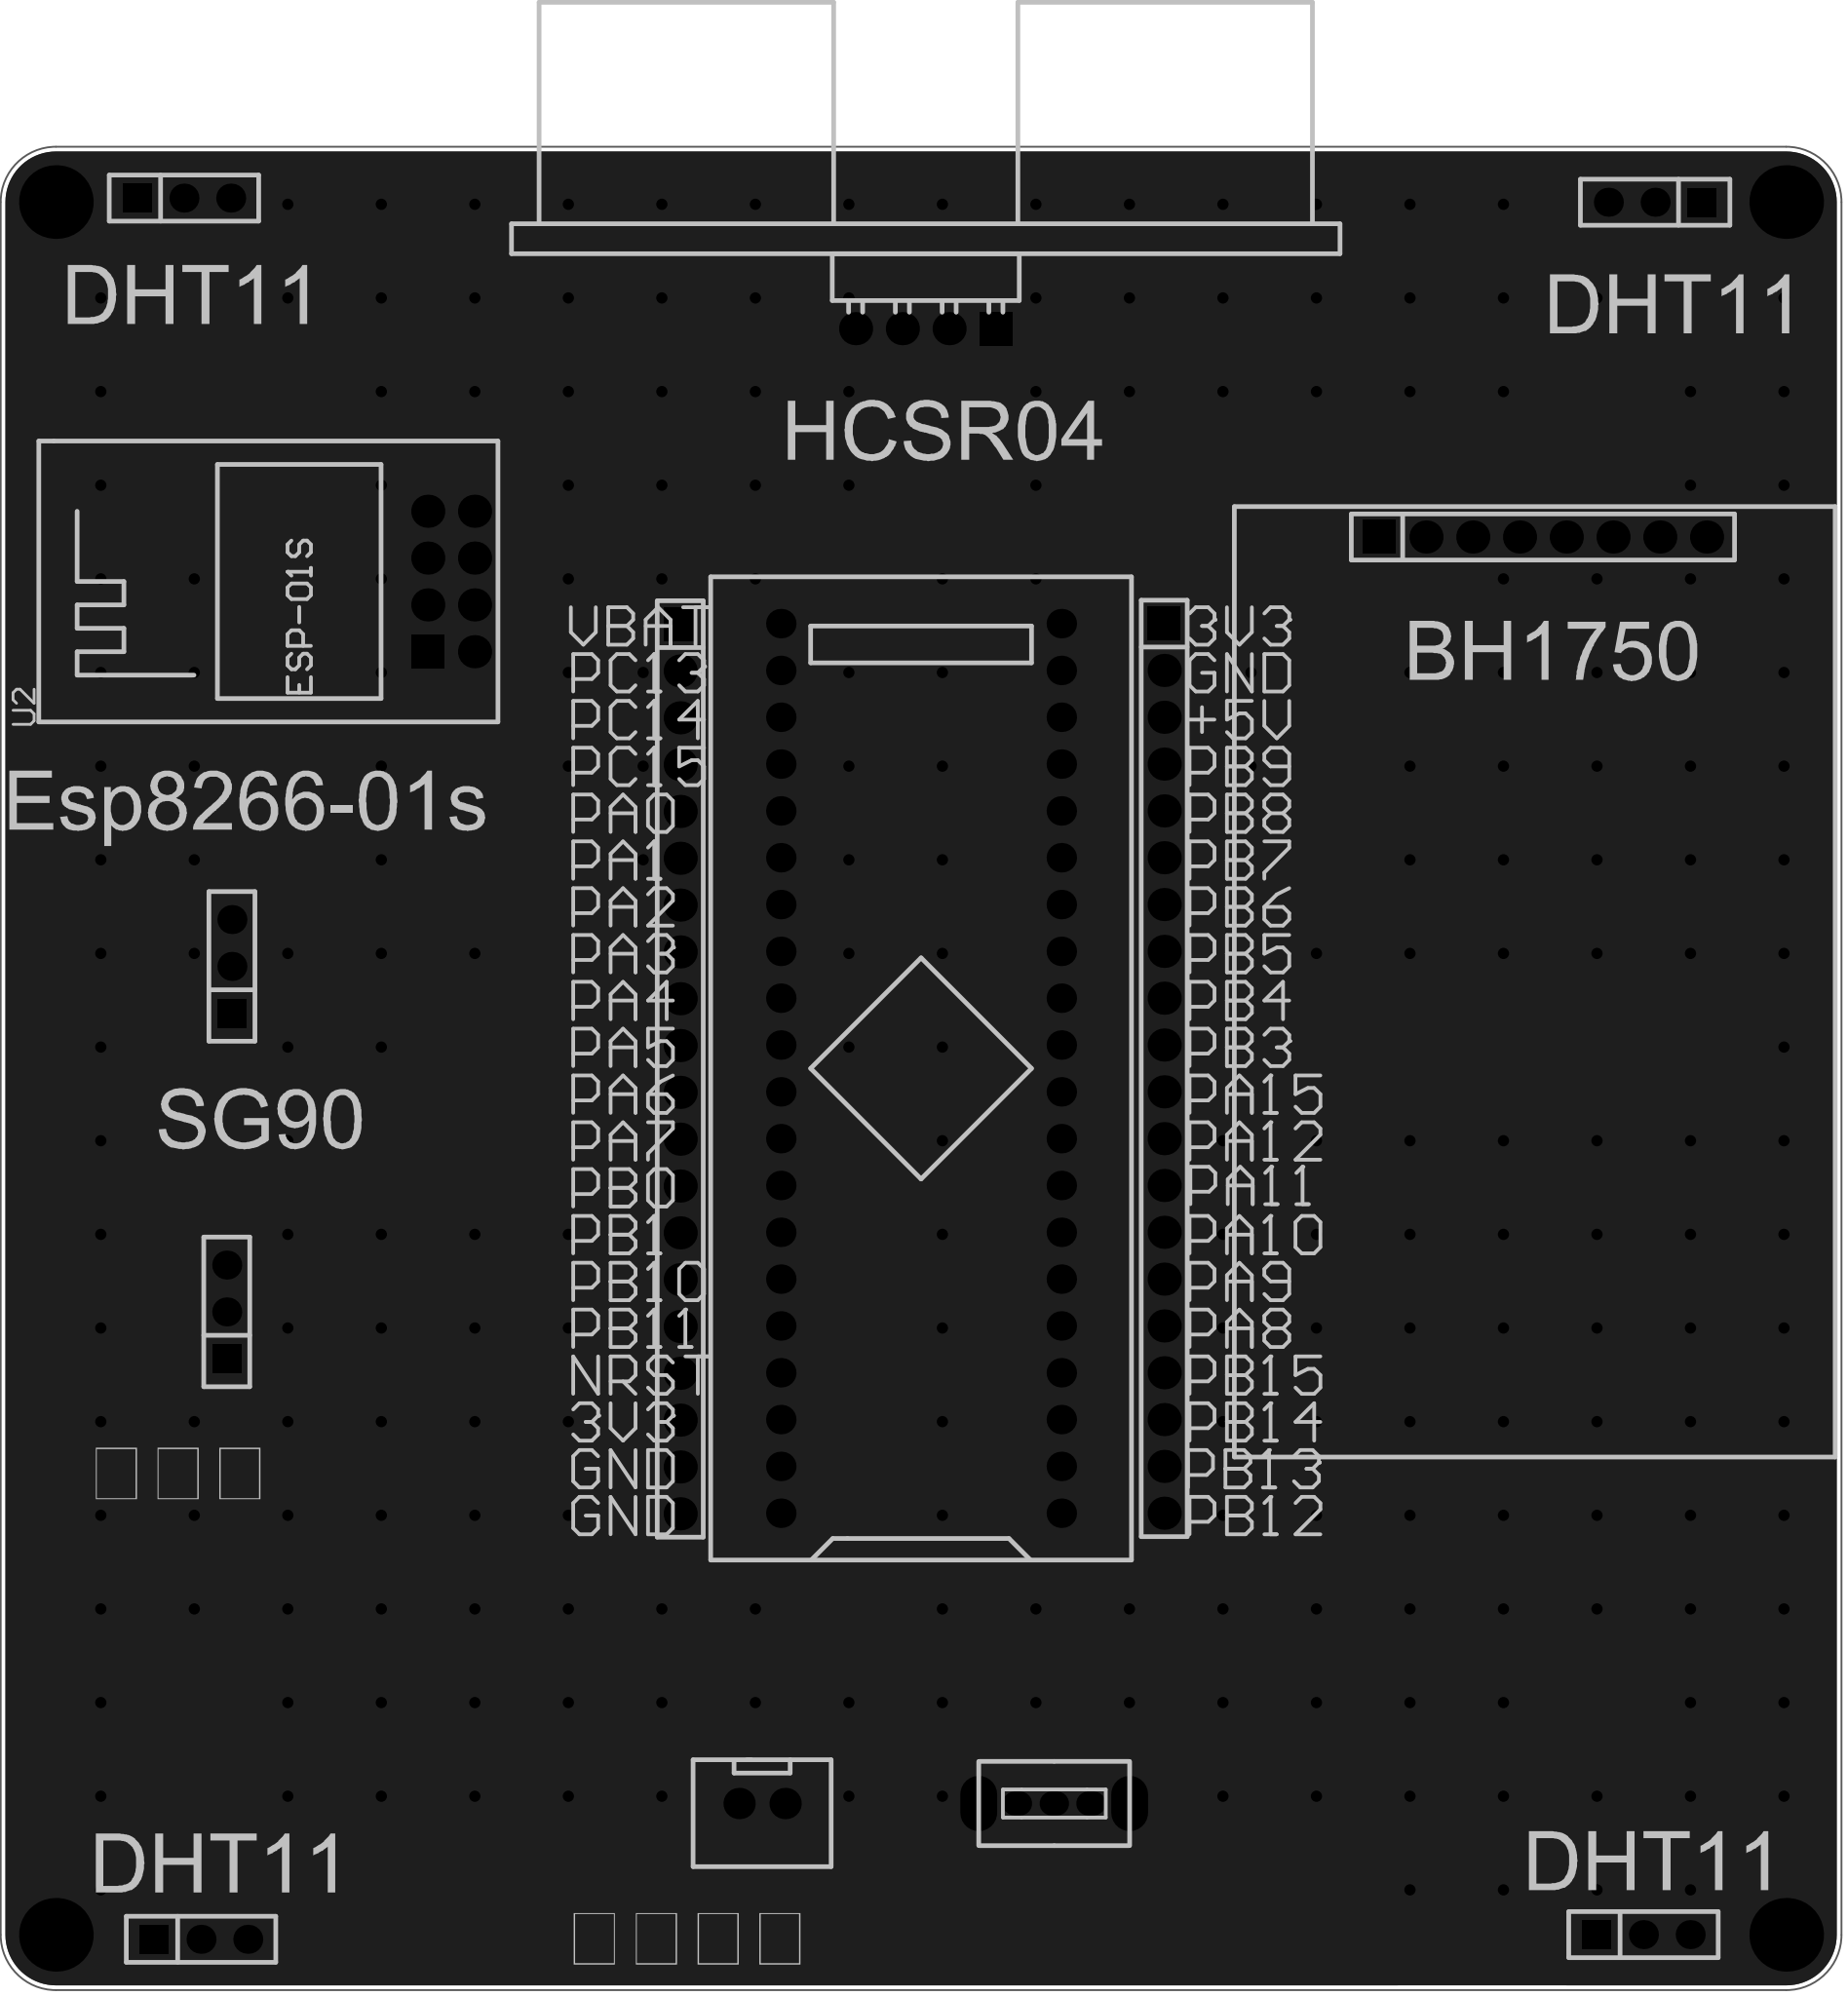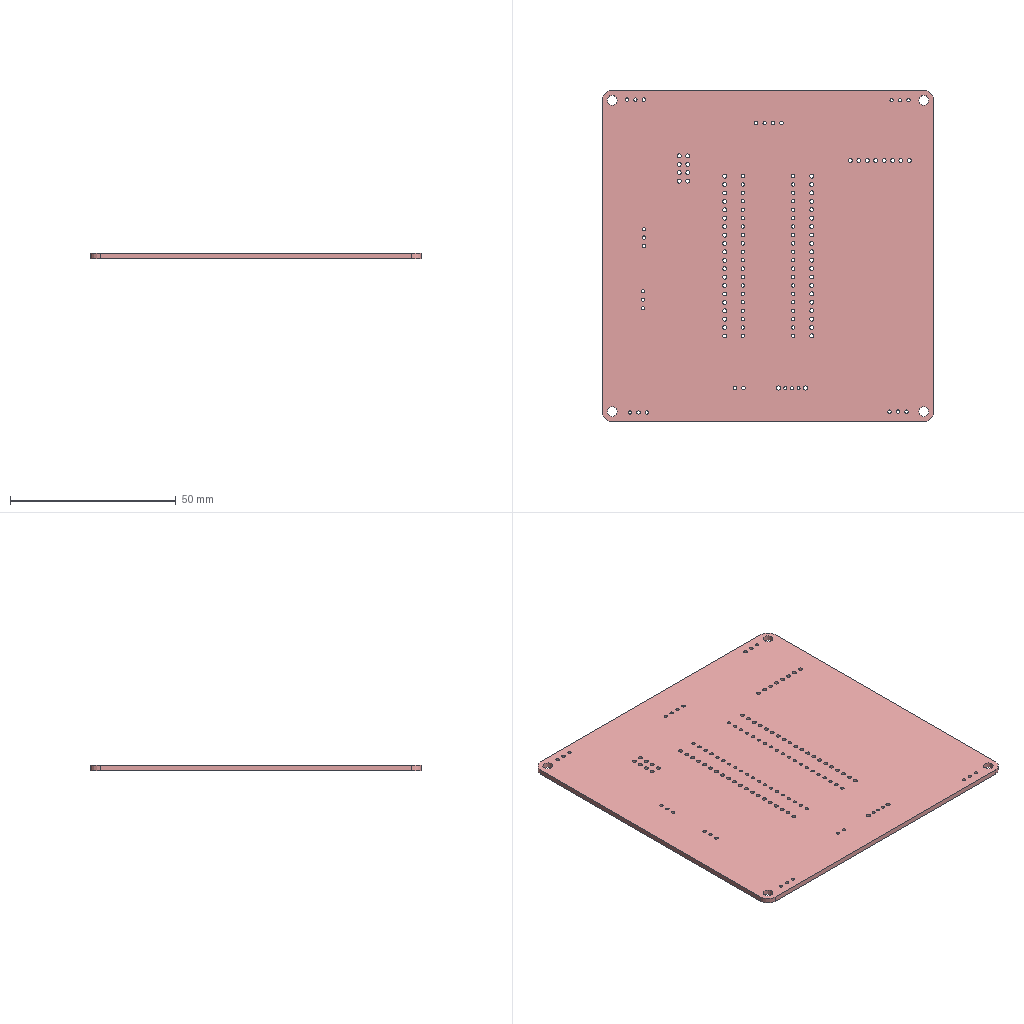Circuit board layout | Altium Designer | box 100 x 100 x 1.6 mm
Layer stack:
# Altium Designer layer stack of  (unit mm; dielectric type: 0 none, 1 core, 2 prepreg, 3 surface material)
index,name,kind,layer,copper_thickness_mm,dielectric_type,dielectric_thickness_mm,dielectric_material,dielectric_constant
0,Top Paste Mask Layer,other,,,,,,
1,Top Silkscreen Layer,other,,,,,,
2,Top Solder Mask Layer,dielectric,,,3,0.01,,3.3
3,Top Layer,copper,Top Layer,0.035,,,,
4,Dielectric1,dielectric,,,3,1.51,FR4,4.5
5,Bottom Layer,copper,Bottom Layer,0.035,,,,
6,Bottom Solder Mask Layer,dielectric,,,3,0.01,,3.3
7,Bottom Silkscreen Layer,other,,,,,,
8,Bottom Paste Mask Layer,other,,,,,,
# drill layer pairs: low layer,high layer
drill_pair,Top Layer,Bottom Layer
Part placement:
Designator,Comment,Layer,Footprint,Center-X(mm),Center-Y(mm),Rotation
U1,STM32F103C8T6-Card,TopLayer,CONN-TH_L53.3-W22.9_STM32F103C8T6-CARD,141.351,130.937,90
CN4,XH2.54*2P_直插,TopLayer,CONN-TH_2P-P2.50-XH2.54-2P,132.715,91.059,0
SW5,,TopLayer,拨动开关,148.582,91.059,180
H1,,TopLayer,HDR-TH_3P-P2.54-V-F,103.632,117.729,90
H3,,TopLayer,HDR-TH_3P-P2.54-V-F,181.229,177.927,180
U2,ESP-01S,TopLayer,WIFIM-TH_ESP-01S,115.824,157.353,90
H2,,TopLayer,HDR-TH_3P-P2.54-V-F,180.594,83.947,0
H4,,TopLayer,HDR-TH_3P-P2.54-V-F,101.307,178.151,0
U3,HC-SR04,TopLayer,TH_HC-SR04V,141.605,171.069,180
H5,,TopLayer,HDR-TH_8P-P2.54-V-F-1,175.133,159.766,0
H7,,TopLayer,HDR-TH_3P-P2.54-V-F,102.235,83.693,0
H8,,TopLayer,HDR-TH_3P-P2.54-V-F,103.912,136.472,90
H6,,TopLayer,HDR-TH_20P-P2.54-V-M-1,128.267,130.907,270
H9,,TopLayer,HDR-TH_20P-P2.54-V-M-1,154.559,130.937,270
Pad and via stacks:
# Altium Designer via and pad stacks of  (unit mm). Each distinct definition once, with the count of objects using it.
# via: kind,start_layer,end_layer,hole_mm,diameter_mm,mode(0 simple;1 top-mid-bottom;2 full stack),diameter_per_layer,count,example_net
# pad: kind,layer,hole_mm,hole_type(0 round;1 square;2 slot),plating,top_size,top_shape(1 round;2 rect;3 octagon;9 rounded rect),mid_size,bottom_size,mode,footprint,size_per_layer,count,example
pad,Multi-Layer,3,0,plated,4x4,1,4x4,4x4,0,,,4,1
pad,Multi-Layer,1,0,plated,1.6x1.6,1,1.6x1.6,1.6x1.6,0,CONN-TH_L53.3-W22.9_STM32F103C8T6-CARD,,40,U1.1
pad,Multi-Layer,1.05,0,plated,1.7x1.7,1,1.7x1.7,1.7x1.7,0,CONN-TH_2P-P2.50-XH2.54-2P,,2,CN4.2
pad,Multi-Layer,0.8992,0,plated,1.6x1.3,1,1.6x1.3,1.6x1.3,0,\u00B2\u00A6\u00B6\u00AF\u00BF\u00AA\u00B9\u00D8,,3,SW5.1
pad,Multi-Layer,1.3,0,plated,3x1.999,1,3x1.999,3x1.999,0,\u00B2\u00A6\u00B6\u00AF\u00BF\u00AA\u00B9\u00D8,,2,SW5.4
pad,Multi-Layer,1.02,0,plated,1.575x1.575,1,1.575x1.575,1.575x1.575,0,HDR-TH_3P-P2.54-V-F,,12,H1.3
pad,Multi-Layer,1.02,0,plated,1.575x1.575,2,1.575x1.575,1.575x1.575,0,HDR-TH_3P-P2.54-V-F,,6,H1.1
pad,Multi-Layer,1.2,0,plated,1.8x1.8,2,1.8x1.8,1.8x1.8,0,WIFIM-TH_ESP-01S,,1,U2.1
pad,Multi-Layer,1.2,0,plated,1.8x1.8,1,1.8x1.8,1.8x1.8,0,WIFIM-TH_ESP-01S,,7,U2.2
pad,Multi-Layer,1.001,0,plated,1.8x1.8,1,1.8x1.8,1.8x1.8,0,TH_HC-SR04V,,3,U3.4
pad,Multi-Layer,1.001,0,plated,1.8x1.8,2,1.8x1.8,1.8x1.8,0,TH_HC-SR04V,,1,U3.1
pad,Multi-Layer,1.2,0,plated,1.8x1.8,2,1.8x1.8,1.8x1.8,0,HDR-TH_8P-P2.54-V-F-1,,1,H5.1
pad,Multi-Layer,1.2,0,plated,1.8x1.8,1,1.8x1.8,1.8x1.8,0,HDR-TH_8P-P2.54-V-F-1,,7,H5.2
pad,Multi-Layer,1.2,0,plated,1.8x1.8,1,1.8x1.8,1.8x1.8,0,HDR-TH_20P-P2.54-V-M-1,,38,H6.20
pad,Multi-Layer,1.2,0,plated,1.8x1.8,2,1.8x1.8,1.8x1.8,0,HDR-TH_20P-P2.54-V-M-1,,2,H6.1
via,Top Layer,Bottom Layer,0.3048,0.61,0,,241,GND
Copper pours:
name,layer,net,type(0 solid;1 hatched;2 none)
Bottom Layer-GND,Bottom Layer,GND,0
Top Layer-GND,Top Layer,GND,0